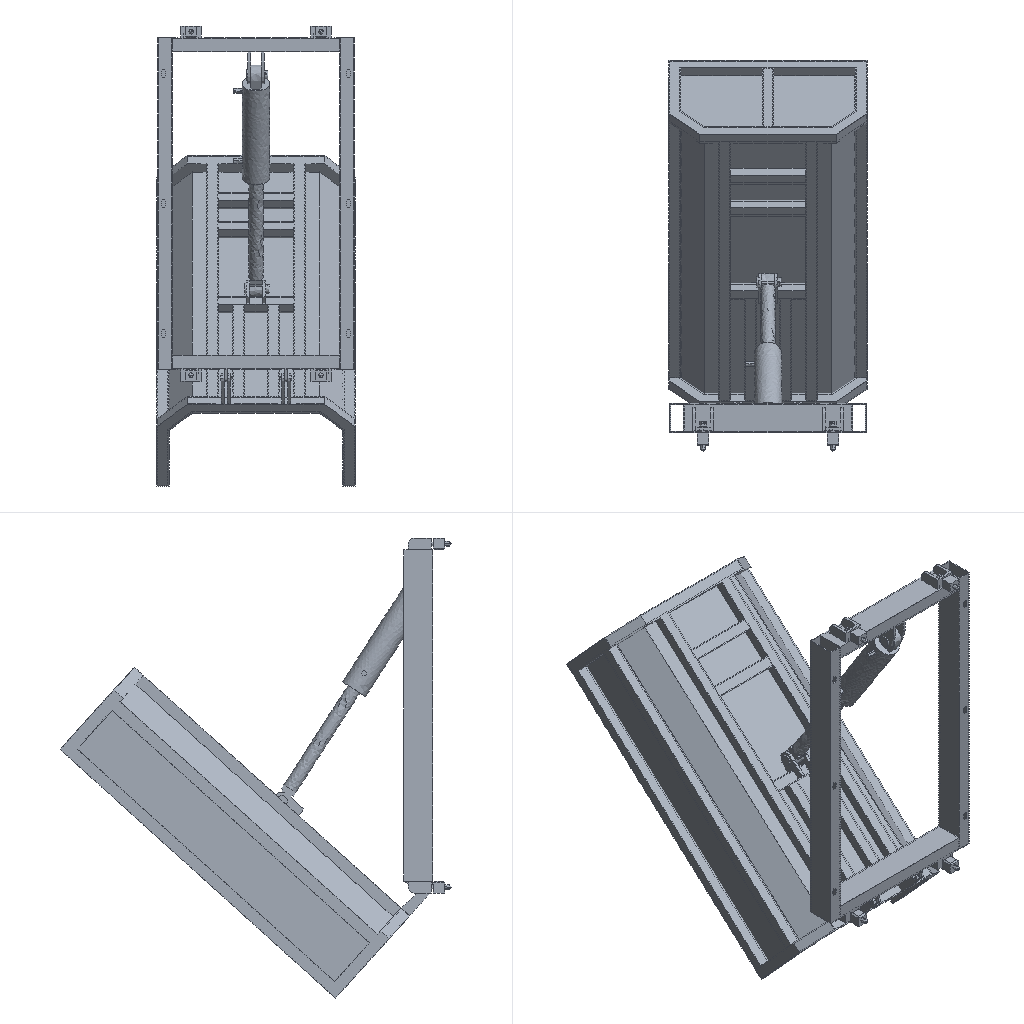Simulation study | ansys workbench
Ansys APDL input file, long lists of numbers shortened:
/batch
/config,noeldb,1     ! force off writing results to database
*get,_wallstrt,active,,time,wall
! ANSYS input file written by Workbench version 2022 R1
! File used for geometry attach:
/title,wbnew--____ (B5)
! ****** Begin Custom Load Command Snippet ******
/COM, ACT Extensions:
/COM,     LSDYNA, 2021.1
/COM,
! ****** End   Custom Load Command Snippet ******
*DIM,_wb_ProjectScratch_dir,string,248
_wb_ProjectScratch_dir(1) = ''
*DIM,_wb_SolverFiles_dir,string,248
_wb_SolverFiles_dir(1) = ''
*DIM,_wb_userfiles_dir,string,248
_wb_userfiles_dir(1) = ''
/com,--- Data in consistent NMM units. See Solving Units in the help system for more information.
/units,MPA
/nopr
/wb,file,start              !  signify a WB generated input file
/prep7
! Turn off shape checking because checks already performed inside WB mesher.
! See help system for more information.
SHPP,OFF,,NOWARN
/nolist
etcon,set             ! allow ANSYS to choose best KEYOP's for 180x elements, resets any applicable keyopt to MAPDL defaults
/com,*********** Nodes for the whole assembly ***********
nblock,3,,401288
(1i9,3e20.9e3)
        1    -4.488006712E+02    -2.775000000E+01    -1.160000000E+03
! (364807 more lines like these left out)
-1
/wb,elem,start            !  set before creation of elements
/com,*********** Elements for Body 1 "__\____-____1" ***********
et,1,186
keyo,1,2,1          ! set full integration on SOLID186
eblock,19,solid,,13612
(19i9)
        1        1        1        1        0        0        0        0       20        0     1952    23088    23089    26138    26139    25938    25937    29030    29029
! (27223 more lines like these left out)
-1
/com,*********** Elements for Body 2 "40X3_______3c_____3e_\__________________(gb t6728-2002) 40__3(1)[3]" ***********
et,2,187
eblock,19,solid,,70641
(19i9)
        2        2        2        2        0        0        0        0       10        0    69359   218340   230217   218664   224153   260977   263721   260972   260975
! (141281 more lines like these left out)
-1
/com,*********** Elements for Body 3 "____\____1" ***********
et,3,186
keyo,3,2,1          ! set full integration on SOLID186
eblock,19,solid,,32
(19i9)
        3        3        3        3        0        0        0        0       20        0   140064   357187   357188   357190   357189   357230   357237   357227   357228
! (63 more lines like these left out)
-1
/com,*********** Elements for Body 4 "____\____1" ***********
et,4,186
keyo,4,2,1          ! set full integration on SOLID186
eblock,19,solid,,32
(19i9)
        4        4        4        4        0        0        0        0       20        0   140000   356579   356580   356582   356581   356622   356629   356619   356620
! (63 more lines like these left out)
-1
/com,*********** Elements for Body 5 "____\____1" ***********
et,5,186
keyo,5,2,1          ! set full integration on SOLID186
eblock,19,solid,,32
(19i9)
        5        5        5        5        0        0        0        0       20        0   140032   356883   356884   356886   356885   356926   356933   356923   356924
! (63 more lines like these left out)
-1
! (35 more sections like these left out)
/wb,elem,end               !  done creating elements
/com,*********** Send User Defined Coordinate System(s) ***********
csys,0
toffst,273.15,  ! Temperature offset from absolute zero
/com,*********** Set Reference Temperature ***********
tref,22.
/wb,mat,start              !  starting to send materials
/com,*********** Send Materials ***********
Temperature = 'TEMP' ! Temperature
MP,DENS,1,7.85e-09,	! tonne mm^-3
MP,ALPX,1,1.2e-05,	! C^-1
MP,C,1,434000000,	! mm^2 s^-2 C^-1
MP,KXX,1,60.5,	! tonne mm s^-3 C^-1
MP,RSVX,1,0.00017,	! ohm mm
MP,EX,1,200000,	! tonne s^-2 mm^-1
MP,NUXY,1,0.3,
MP,MURX,1,10000,
Temperature = 'TEMP' ! Temperature
MP,DENS,2,7.85e-09,	! tonne mm^-3
MP,ALPX,2,1.2e-05,	! C^-1
MP,C,2,434000000,	! mm^2 s^-2 C^-1
MP,KXX,2,60.5,	! tonne mm s^-3 C^-1
MP,RSVX,2,0.00017,	! ohm mm
MP,EX,2,200000,	! tonne s^-2 mm^-1
MP,NUXY,2,0.3,
MP,MURX,2,10000,
Temperature = 'TEMP' ! Temperature
MP,DENS,3,7.85e-09,	! tonne mm^-3
MP,ALPX,3,1.2e-05,	! C^-1
MP,C,3,434000000,	! mm^2 s^-2 C^-1
MP,KXX,3,60.5,	! tonne mm s^-3 C^-1
MP,RSVX,3,0.00017,	! ohm mm
MP,EX,3,200000,	! tonne s^-2 mm^-1
MP,NUXY,3,0.3,
MP,MURX,3,10000,
Temperature = 'TEMP' ! Temperature
MP,DENS,4,7.85e-09,	! tonne mm^-3
MP,ALPX,4,1.2e-05,	! C^-1
MP,C,4,434000000,	! mm^2 s^-2 C^-1
MP,KXX,4,60.5,	! tonne mm s^-3 C^-1
MP,RSVX,4,0.00017,	! ohm mm
MP,EX,4,200000,	! tonne s^-2 mm^-1
MP,NUXY,4,0.3,
MP,MURX,4,10000,
Temperature = 'TEMP' ! Temperature
MP,DENS,5,7.85e-09,	! tonne mm^-3
MP,ALPX,5,1.2e-05,	! C^-1
MP,C,5,434000000,	! mm^2 s^-2 C^-1
MP,KXX,5,60.5,	! tonne mm s^-3 C^-1
MP,RSVX,5,0.00017,	! ohm mm
MP,EX,5,200000,	! tonne s^-2 mm^-1
MP,NUXY,5,0.3,
MP,MURX,5,10000,
Temperature = 'TEMP' ! Temperature
MP,DENS,6,7.85e-09,	! tonne mm^-3
MP,ALPX,6,1.2e-05,	! C^-1
MP,C,6,434000000,	! mm^2 s^-2 C^-1
MP,KXX,6,60.5,	! tonne mm s^-3 C^-1
MP,RSVX,6,0.00017,	! ohm mm
MP,EX,6,200000,	! tonne s^-2 mm^-1
MP,NUXY,6,0.3,
MP,MURX,6,10000,
Temperature = 'TEMP' ! Temperature
MP,DENS,7,7.85e-09,	! tonne mm^-3
MP,ALPX,7,1.2e-05,	! C^-1
MP,C,7,434000000,	! mm^2 s^-2 C^-1
MP,KXX,7,60.5,	! tonne mm s^-3 C^-1
MP,RSVX,7,0.00017,	! ohm mm
MP,EX,7,200000,	! tonne s^-2 mm^-1
MP,NUXY,7,0.3,
MP,MURX,7,10000,
Temperature = 'TEMP' ! Temperature
MP,DENS,8,7.85e-09,	! tonne mm^-3
MP,ALPX,8,1.2e-05,	! C^-1
MP,C,8,434000000,	! mm^2 s^-2 C^-1
MP,KXX,8,60.5,	! tonne mm s^-3 C^-1
MP,RSVX,8,0.00017,	! ohm mm
MP,EX,8,200000,	! tonne s^-2 mm^-1
MP,NUXY,8,0.3,
MP,MURX,8,10000,
Temperature = 'TEMP' ! Temperature
MP,DENS,9,7.85e-09,	! tonne mm^-3
MP,ALPX,9,1.2e-05,	! C^-1
MP,C,9,434000000,	! mm^2 s^-2 C^-1
MP,KXX,9,60.5,	! tonne mm s^-3 C^-1
MP,RSVX,9,0.00017,	! ohm mm
MP,EX,9,200000,	! tonne s^-2 mm^-1
! (281 more lines like these left out)
/wb,mat,end                !  done sending materials
!************************* Model Summary ********************
!__\____-____1,	结构钢,	matid,	1
!40X3_______3c_____3e_\__________________(gb t6728-2002) 40__3(1)[3],	结构钢,	matid,	2
!____\____1,	结构钢,	matid,	3
! (39 more lines like these left out)
*get,_xmin,node,,mnloc,x
*get,_ymin,node,,mnloc,y
*get,_zmin,node,,mnloc,z
*get,_xmax,node,,mxloc,x
*get,_ymax,node,,mxloc,y
*get,_zmax,node,,mxloc,z
_ASMDIAG=(_xmax-_xmin)*(_xmax-_xmin)+(_ymax-_ymin)*(_ymax-_ymin)+(_zmax-_zmin)*(_zmax-_zmin)
_ASMDIAG=SQRT(_ASMDIAG)
/wb,contact,start          !  starting to send contact
/com,*********** Create Contact "接触区域" ***********
/com,            Real Constant Set For Above Contact Is 42 & 41
*set,tid,42
*set,cid,41
r,tid
r,cid
et,tid,170
et,cid,174
eblock,10,,,6652
(15i9)
   258682       42       42       42        0    15307    12437    12355    12354    40899    40735    40732    40733
! (6651 more lines like these left out)
-1
eblock,10,,,6652
(15i9)
   265334       41       41       41        0    15307    12437    12355    12354    40899    40735    40732    40733
! (6651 more lines like these left out)
-1
eblock,10,,,6606
(15i9)
   271986       41       42       41        0   230850   231170   231390   231390   332666   334211   231390   332669
! (6605 more lines like these left out)
-1
eblock,10,,,6606
(15i9)
   278592       42       41       42        0   230850   231170   231390   231390   332666   334211   231390   332669
! (6605 more lines like these left out)
-1
keyo,cid,8,2               ! auto create asymmetric contact (from Program Controlled setting)
keyo,cid,10,0              ! adjust contact stiffness each NR iteration (from Program Controlled setting)
keyo,cid,12,5              ! bonded always
keyo,cid,2,2               ! MPC contact.  Valid only for bonded or no separation.  Requires nodal detection
keyo,cid,4,2               ! on nodal point - normal to target surface (from Program Controlled setting)
keyo,cid,9,1               ! ignore initial gaps/penetration
keyo,cid,7,0               ! No Prediction
rmod,tid,3,10.      ! FKN
rmod,tid,5,0.       ! ICONT
rmod,tid,6,0.       ! PINB
rmod,tid,10,0.      ! CNOF
rmod,tid,12,0.      ! FKT
rmod,tid,36,143     ! WB DSID
rmod,cid,3,10.      ! FKN
rmod,cid,5,0.       ! ICONT
rmod,cid,6,0.       ! PINB
rmod,cid,10,0.      ! CNOF
rmod,cid,12,0.      ! FKT
rmod,cid,36,143     ! WB DSID
/com,*********** Create Contact "接触区域 2" ***********
/com,            Real Constant Set For Above Contact Is 44 & 43
*set,tid,44
*set,cid,43
r,tid
r,cid
et,tid,170
et,cid,174
eblock,10,,,164
(15i9)
   285198       44       44       44        0    12076    12075    12134    12133    40064    40065    40209    40068
! (163 more lines like these left out)
-1
eblock,10,,,164
(15i9)
   285362       43       43       43        0    12076    12075    12134    12133    40064    40065    40209    40068
! (163 more lines like these left out)
-1
eblock,10,,,288
(15i9)
   285526       43       44       43        0     3978     4081     4093     4082     8095     8315     8318     8096
! (287 more lines like these left out)
-1
eblock,10,,,288
(15i9)
   285814       44       43       44        0     3978     4081     4093     4082     8095     8315     8318     8096
! (287 more lines like these left out)
-1
keyo,cid,8,2               ! auto create asymmetric contact (from Program Controlled setting)
keyo,cid,10,0              ! adjust contact stiffness each NR iteration (from Program Controlled setting)
keyo,cid,12,5              ! bonded always
keyo,cid,2,2               ! MPC contact.  Valid only for bonded or no separation.  Requires nodal detection
keyo,cid,4,2               ! on nodal point - normal to target surface (from Program Controlled setting)
keyo,cid,9,1               ! ignore initial gaps/penetration
keyo,cid,7,0               ! No Prediction
rmod,tid,3,10.      ! FKN
rmod,tid,5,0.       ! ICONT
rmod,tid,6,0.       ! PINB
rmod,tid,10,0.      ! CNOF
rmod,tid,12,0.      ! FKT
rmod,tid,36,146     ! WB DSID
rmod,cid,3,10.      ! FKN
rmod,cid,5,0.       ! ICONT
rmod,cid,6,0.       ! PINB
rmod,cid,10,0.      ! CNOF
rmod,cid,12,0.      ! FKT
rmod,cid,36,146     ! WB DSID
/com,*********** Create Contact "接触区域 3" ***********
/com,            Real Constant Set For Above Contact Is 46 & 45
*set,tid,46
*set,cid,45
r,tid
r,cid
et,tid,170
et,cid,174
eblock,10,,,164
(15i9)
   286102       46       46       46        0    12076    12075    12134    12133    40064    40065    40209    40068
! (163 more lines like these left out)
-1
eblock,10,,,164
(15i9)
   286266       45       45       45        0    12076    12075    12134    12133    40064    40065    40209    40068
! (163 more lines like these left out)
-1
eblock,10,,,321
(15i9)
   286430       45       46       45        0   119141   119211   119359   119359   135857   136277   119359   135860
! (320 more lines like these left out)
-1
eblock,10,,,321
(15i9)
   286751       46       45       46        0   119141   119211   119359   119359   135857   136277   119359   135860
! (320 more lines like these left out)
-1
keyo,cid,8,2               ! auto create asymmetric contact (from Program Controlled setting)
keyo,cid,10,0              ! adjust contact stiffness each NR iteration (from Program Controlled setting)
keyo,cid,12,5              ! bonded always
keyo,cid,2,2               ! MPC contact.  Valid only for bonded or no separation.  Requires nodal detection
keyo,cid,4,2               ! on nodal point - normal to target surface (from Program Controlled setting)
keyo,cid,9,1               ! ignore initial gaps/penetration
keyo,cid,7,0               ! No Prediction
rmod,tid,3,10.      ! FKN
rmod,tid,5,0.       ! ICONT
rmod,tid,6,0.       ! PINB
rmod,tid,10,0.      ! CNOF
rmod,tid,12,0.      ! FKT
rmod,tid,36,149     ! WB DSID
rmod,cid,3,10.      ! FKN
rmod,cid,5,0.       ! ICONT
rmod,cid,6,0.       ! PINB
rmod,cid,10,0.      ! CNOF
rmod,cid,12,0.      ! FKT
rmod,cid,36,149     ! WB DSID
/com,*********** Create Contact "接触区域 6" ***********
/com,            Real Constant Set For Above Contact Is 48 & 47
*set,tid,48
*set,cid,47
r,tid
r,cid
et,tid,170
et,cid,174
eblock,10,,,26
(15i9)
   287072       48       48       48        0   226935   227558   227524   227524   316348   318501   227524   316346
! (25 more lines like these left out)
-1
eblock,10,,,26
(15i9)
   287098       47       47       47        0   226935   227558   227524   227524   316348   318501   227524   316346
! (25 more lines like these left out)
-1
eblock,10,,,3
(15i9)
   287124       47       48       47        0   357220   357219   357198   357197   357424   357393   357390   357391
   287125       47       48       47        0   357219   357218   357199   357198   357423   357395   357392   357393
   287126       47       48       47        0   357218   357217   357200   357199   357422   357397   357394   357395
-1
eblock,10,,,3
(15i9)
   287127       48       47       48        0   357220   357219   357198   357197   357424   357393   357390   357391
   287128       48       47       48        0   357219   357218   357199   357198   357423   357395   357392   357393
   287129       48       47       48        0   357218   357217   357200   357199   357422   357397   357394   357395
-1
keyo,cid,8,2               ! auto create asymmetric contact (from Program Controlled setting)
keyo,cid,10,0              ! adjust contact stiffness each NR iteration (from Program Controlled setting)
keyo,cid,12,5              ! bonded always
keyo,cid,2,2               ! MPC contact.  Valid only for bonded or no separation.  Requires nodal detection
keyo,cid,4,2               ! on nodal point - normal to target surface (from Program Controlled setting)
keyo,cid,9,1               ! ignore initial gaps/penetration
keyo,cid,7,0               ! No Prediction
rmod,tid,3,10.      ! FKN
rmod,tid,5,0.       ! ICONT
rmod,tid,6,0.       ! PINB
rmod,tid,10,0.      ! CNOF
rmod,tid,12,0.      ! FKT
rmod,tid,36,158     ! WB DSID
rmod,cid,3,10.      ! FKN
rmod,cid,5,0.       ! ICONT
rmod,cid,6,0.       ! PINB
rmod,cid,10,0.      ! CNOF
rmod,cid,12,0.      ! FKT
rmod,cid,36,158     ! WB DSID
/com,*********** Create Contact "接触区域 7" ***********
/com,            Real Constant Set For Above Contact Is 50 & 49
*set,tid,50
*set,cid,49
r,tid
r,cid
et,tid,170
et,cid,174
eblock,10,,,26
(15i9)
   287130       50       50       50        0   216992   216993   226941   226941   249573   249585   226941   249577
! (25 more lines like these left out)
-1
eblock,10,,,26
(15i9)
   287156       49       49       49        0   216992   216993   226941   226941   249573   249585   226941   249577
! (25 more lines like these left out)
-1
eblock,10,,,3
(15i9)
   287182       49       50       49        0   356612   356611   356590   356589   356816   356785   356782   356783
   287183       49       50       49        0   356611   356610   356591   356590   356815   356787   356784   356785
   287184       49       50       49        0   356610   356609   356592   356591   356814   356789   356786   356787
-1
eblock,10,,,3
(15i9)
   287185       50       49       50        0   356612   356611   356590   356589   356816   356785   356782   356783
   287186       50       49       50        0   356611   356610   356591   356590   356815   356787   356784   356785
   287187       50       49       50        0   356610   356609   356592   356591   356814   356789   356786   356787
-1
keyo,cid,8,2               ! auto create asymmetric contact (from Program Controlled setting)
keyo,cid,10,0              ! adjust contact stiffness each NR iteration (from Program Controlled setting)
keyo,cid,12,5              ! bonded always
keyo,cid,2,2               ! MPC contact.  Valid only for bonded or no separation.  Requires nodal detection
keyo,cid,4,2               ! on nodal point - normal to target surface (from Program Controlled setting)
keyo,cid,9,1               ! ignore initial gaps/penetration
keyo,cid,7,0               ! No Prediction
rmod,tid,3,10.      ! FKN
rmod,tid,5,0.       ! ICONT
rmod,tid,6,0.       ! PINB
rmod,tid,10,0.      ! CNOF
rmod,tid,12,0.      ! FKT
rmod,tid,36,161     ! WB DSID
rmod,cid,3,10.      ! FKN
rmod,cid,5,0.       ! ICONT
rmod,cid,6,0.       ! PINB
rmod,cid,10,0.      ! CNOF
rmod,cid,12,0.      ! FKT
rmod,cid,36,161     ! WB DSID
! (53 more sections like these left out)
/wb,contact,end            !  done creating contacts
/golist
/wb,load,start             !  starting to send loads
/com,*********** Fixed Supports ***********
CMBLOCK,_FIXEDSU,NODE,      148
(8i10)
    360371    360372    360373    360374    360375    360376    360377    360378
! (18 more lines like these left out)
cmsel,s,_FIXEDSU
d,all,all
nsel,all
/com,*********** Define Force Using Surface Effect Elements ***********
local,12,0,0.,0.,0.,0.,0.,0.
csys,0
et,157,154
eblock,10,,,7636
(15i9)
   298150      157      157      157       12    30350    29120    29038    29037    87593    87429    87426    87427
! (7635 more lines like these left out)
-1
esel,s,type,,157
keyop,157,2,1                ! Apply load in local coordinate system
keyop,157,7,1                ! Use original area so load is constant in large deformation
esel,all
/gst,on,on
fini
*get,_numnode,node,0,count
*get,_numelem,elem,0,count
*get, _MAXELEMNUM, elem, 0, NUM, MAX
*get, _MAXNODENUM, node, 0, NUM, MAX
*get, _MAXELEMTYPE, etyp, 0, NUM, MAX
*get, _MAXREALCONST, real, 0, NUM, MAX
/go
/wb,load,end               !  done creating loads
/com,--- Number of total nodes = %_numnode%
/com,--- Number of contact elements = 47104
/com,--- Number of spring elements = 0
/com,--- Number of bearing elements = 0
/com,--- Number of solid elements = 142657
/com,--- Number of condensed parts = 0
/com,--- Number of total elements = %_numelem%
*get,_wallbsol,active,,time,wall
/com,****************************************************************************
/com,*************************    SOLUTION       ********************************
/com,****************************************************************************
/solu
antype,0                   ! static analysis
neqit,1,force              ! Force 1 eq iteration since only nonlinearity is bonded/no sep contact
pred,off
_thickRatio=0.025   ! Ratio of thick parts in the model
eqsl,sparse,,,,,1
cntr,print,1               ! print out contact info and also make no initial contact an error
dmpoption,emat,no             ! Don't combine emat file for DANSYS
dmpoption,esav,no             ! Don't combine esav file for DANSYS
nldiag,cont,iter           ! print out contact info each equilibrium iteration
rescontrol,,none                 ! Do not keep any restart files
/com,****************************************************
/com,******************* SOLVE FOR LS 1 OF 1 ****************
esel,s,type,,157
nsle
sfe,all,1,pres,1,0.
sfe,all,2,pres,1,-6.04220466096275e-003
sfe,all,3,pres,1,5.18931354352186e-035
nsel,all
esel,all
/nopr
/gopr
nsub,1,1,1
time,1.
outres,erase
outres,all,none
outres,nsol,all,
outres,rsol,all
outres,eangl,all
outres,etmp,all
outres,veng,all
outres,strs,all,
outres,epel,all,
outres,eppl,all,
outres,cont,all,
! *********** WB SOLVE COMMAND ***********
! check interactive state
*get,ANSINTER_,active,,int
*if,ANSINTER_,ne,0,then
/eof
*endif
solve
/com *************** Write FE CONNECTORS *********
CEWRITE,file,ce,,INTE
/com,****************************************************
/com,*************** FINISHED SOLVE FOR LS 1 *************
*get,_wallasol,active,,time,wall
/nopr
*get,_numnode,node,0,count
*get,_numelem,elem,0,count
*get, _MAXELEMNUM, elem, 0, NUM, MAX
*get, _MAXNODENUM, node, 0, NUM, MAX,,,INTERNAL
*get, _MAXELEMTYPE, etyp, 0, NUM, MAX
*get, _MAXREALCONST, real, 0, NUM, MAX
/gopr
/post1
xmlo,ENCODING,ISO-8859-1
xmlo,parm
/xml,parm,xml
fini
/gopr
*get,_walldone,active,,time,wall
_preptime=(_wallbsol-_wallstrt)*3600
_solvtime=(_wallasol-_wallbsol)*3600
_posttime=(_walldone-_wallasol)*3600
_totaltim=(_walldone-_wallstrt)*3600
*get,_dlbratio,active,0,solu,dlbr
*get,_combtime,active,0,solu,comb
*get,_ssmode,active,0,solu,ssmm
*get,_ndofs,active,0,solu,ndof
*get,_sol_end_time,active,0,set,time
*if,_sol_end_time,eq,1.,then
/fclean				!clean distributed files
*endif
/com,--- Total number of nodes = %_numnode%
/com,--- Total number of elements = %_numelem%
/com,--- Element load balance ratio = %_dlbratio%
/com,--- Time to combine distributed files = %_combtime%
/com,--- Sparse memory mode = %_ssmode%
/com,--- Number of DOF = %_ndofs%
/wb,file,end               ! done with WB generated input